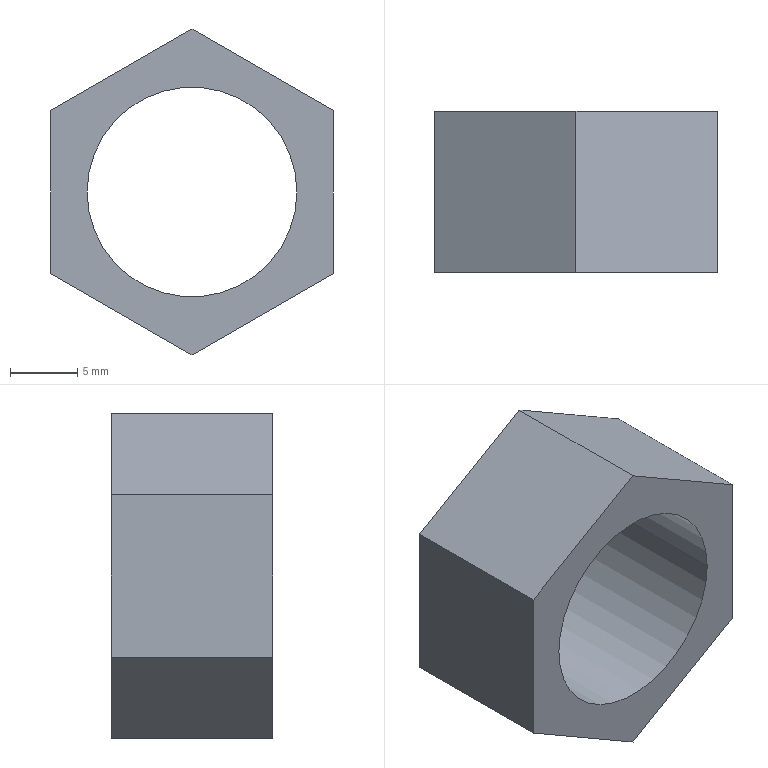Part | STEP file | Scale factor 1[13] | 1 solid | 10 faces | box 21 x 12 x 24.249 mm | volume 2289 mm3 | plane 8 | cylinder 2 | commonest cylinder face diameters 15.6 x2
STEP:
#1=CARTESIAN_POINT('',(-666.538,-401.273,3148.5));
#2=VERTEX_POINT('',#1);
#3=CARTESIAN_POINT('',(-650.938,-401.273,3148.5));
#4=VERTEX_POINT('',#3);
#5=CARTESIAN_POINT('',(-658.738,-401.273,3148.5));
#6=DIRECTION('',(0.,1.,0.));
#7=DIRECTION('',(1.,0.,0.000000001));
#8=AXIS2_PLACEMENT_3D('',#5,#6,#7);
#9=CIRCLE('',#8,7.8);
#10=EDGE_CURVE('',#2,#4,#9,.T.);
#11=ORIENTED_EDGE('',*,*,#10,.T.);
#12=CARTESIAN_POINT('',(-650.938,-413.273,3148.5));
#13=VERTEX_POINT('',#12);
#14=CARTESIAN_POINT('',(-650.938,-401.273,3148.5));
#15=DIRECTION('',(0.,1.,0.));
#16=VECTOR('',#15,1000.);
#17=LINE('',#14,#16);
#18=EDGE_CURVE('',#13,#4,#17,.T.);
#19=ORIENTED_EDGE('',*,*,#18,.F.);
#20=CARTESIAN_POINT('',(-666.538,-413.273,3148.5));
#21=VERTEX_POINT('',#20);
#22=CARTESIAN_POINT('',(-658.738,-413.273,3148.5));
#23=DIRECTION('',(0.,1.,0.));
#24=DIRECTION('',(1.,0.,0.000000001));
#25=AXIS2_PLACEMENT_3D('',#22,#23,#24);
#26=CIRCLE('',#25,7.8);
#27=EDGE_CURVE('',#21,#13,#26,.T.);
#28=ORIENTED_EDGE('',*,*,#27,.F.);
#29=CARTESIAN_POINT('',(-666.538,-401.273,3148.5));
#30=DIRECTION('',(0.,1.,0.));
#31=VECTOR('',#30,1000.);
#32=LINE('',#29,#31);
#33=EDGE_CURVE('',#21,#2,#32,.T.);
#34=ORIENTED_EDGE('',*,*,#33,.T.);
#35=EDGE_LOOP('',(#11,#19,#28,#34));
#36=FACE_OUTER_BOUND('',#35,.T.);
#37=CARTESIAN_POINT('',(-658.738,-401.273,3148.5));
#38=DIRECTION('',(0.,-1.,0.));
#39=DIRECTION('',(1.,0.,0.000000001));
#40=AXIS2_PLACEMENT_3D('',#37,#38,#39);
#41=CYLINDRICAL_SURFACE('',#40,7.8);
#42=ADVANCED_FACE('',(#36),#41,.F.);
#43=CARTESIAN_POINT('',(-648.238,-401.273,3142.438));
#44=VERTEX_POINT('',#43);
#45=CARTESIAN_POINT('',(-658.738,-401.273,3136.376));
#46=VERTEX_POINT('',#45);
#47=CARTESIAN_POINT('',(-648.238,-401.273,3142.438));
#48=DIRECTION('',(-0.866,0.,-0.5));
#49=VECTOR('',#48,1000.);
#50=LINE('',#47,#49);
#51=EDGE_CURVE('',#44,#46,#50,.T.);
#52=ORIENTED_EDGE('',*,*,#51,.T.);
#53=CARTESIAN_POINT('',(-669.238,-401.273,3142.438));
#54=VERTEX_POINT('',#53);
#55=CARTESIAN_POINT('',(-658.738,-401.273,3136.376));
#56=DIRECTION('',(-0.866,0.,0.5));
#57=VECTOR('',#56,1000.);
#58=LINE('',#55,#57);
#59=EDGE_CURVE('',#46,#54,#58,.T.);
#60=ORIENTED_EDGE('',*,*,#59,.T.);
#61=CARTESIAN_POINT('',(-669.238,-401.273,3154.562));
#62=VERTEX_POINT('',#61);
#63=CARTESIAN_POINT('',(-669.238,-401.273,3142.438));
#64=DIRECTION('',(-0.000000001,0.,1.));
#65=VECTOR('',#64,1000.);
#66=LINE('',#63,#65);
#67=EDGE_CURVE('',#54,#62,#66,.T.);
#68=ORIENTED_EDGE('',*,*,#67,.T.);
#69=CARTESIAN_POINT('',(-658.738,-401.273,3160.624));
#70=VERTEX_POINT('',#69);
#71=CARTESIAN_POINT('',(-669.238,-401.273,3154.562));
#72=DIRECTION('',(0.866,0.,0.5));
#73=VECTOR('',#72,1000.);
#74=LINE('',#71,#73);
#75=EDGE_CURVE('',#62,#70,#74,.T.);
#76=ORIENTED_EDGE('',*,*,#75,.T.);
#77=CARTESIAN_POINT('',(-648.238,-401.273,3154.562));
#78=VERTEX_POINT('',#77);
#79=CARTESIAN_POINT('',(-658.738,-401.273,3160.624));
#80=DIRECTION('',(0.866,0.,-0.5));
#81=VECTOR('',#80,1000.);
#82=LINE('',#79,#81);
#83=EDGE_CURVE('',#70,#78,#82,.T.);
#84=ORIENTED_EDGE('',*,*,#83,.T.);
#85=CARTESIAN_POINT('',(-648.238,-401.273,3154.562));
#86=DIRECTION('',(0.000000001,0.,-1.));
#87=VECTOR('',#86,1000.);
#88=LINE('',#85,#87);
#89=EDGE_CURVE('',#78,#44,#88,.T.);
#90=ORIENTED_EDGE('',*,*,#89,.T.);
#91=EDGE_LOOP('',(#52,#60,#68,#76,#84,#90));
#92=FACE_OUTER_BOUND('',#91,.T.);
#93=ORIENTED_EDGE('',*,*,#10,.F.);
#94=CARTESIAN_POINT('',(-658.738,-401.273,3148.5));
#95=DIRECTION('',(0.,1.,0.));
#96=DIRECTION('',(1.,0.,0.000000001));
#97=AXIS2_PLACEMENT_3D('',#94,#95,#96);
#98=CIRCLE('',#97,7.8);
#99=EDGE_CURVE('',#4,#2,#98,.T.);
#100=ORIENTED_EDGE('',*,*,#99,.F.);
#101=EDGE_LOOP('',(#93,#100));
#102=FACE_BOUND('',#101,.T.);
#103=CARTESIAN_POINT('',(-658.738,-401.273,3148.5));
#104=DIRECTION('',(0.,1.,0.));
#105=DIRECTION('',(-1.,0.,-0.000000001));
#106=AXIS2_PLACEMENT_3D('',#103,#104,#105);
#107=PLANE('',#106);
#108=ADVANCED_FACE('',(#92,#102),#107,.T.);
#109=CARTESIAN_POINT('',(-648.238,-413.273,3142.438));
#110=VERTEX_POINT('',#109);
#111=CARTESIAN_POINT('',(-658.738,-413.273,3136.376));
#112=VERTEX_POINT('',#111);
#113=CARTESIAN_POINT('',(-648.238,-413.273,3142.438));
#114=DIRECTION('',(-0.866,0.,-0.5));
#115=VECTOR('',#114,1000.);
#116=LINE('',#113,#115);
#117=EDGE_CURVE('',#110,#112,#116,.T.);
#118=ORIENTED_EDGE('',*,*,#117,.F.);
#119=CARTESIAN_POINT('',(-648.238,-413.273,3154.562));
#120=VERTEX_POINT('',#119);
#121=CARTESIAN_POINT('',(-648.238,-413.273,3154.562));
#122=DIRECTION('',(0.000000001,0.,-1.));
#123=VECTOR('',#122,1000.);
#124=LINE('',#121,#123);
#125=EDGE_CURVE('',#120,#110,#124,.T.);
#126=ORIENTED_EDGE('',*,*,#125,.F.);
#127=CARTESIAN_POINT('',(-658.738,-413.273,3160.624));
#128=VERTEX_POINT('',#127);
#129=CARTESIAN_POINT('',(-658.738,-413.273,3160.624));
#130=DIRECTION('',(0.866,0.,-0.5));
#131=VECTOR('',#130,1000.);
#132=LINE('',#129,#131);
#133=EDGE_CURVE('',#128,#120,#132,.T.);
#134=ORIENTED_EDGE('',*,*,#133,.F.);
#135=CARTESIAN_POINT('',(-669.238,-413.273,3154.562));
#136=VERTEX_POINT('',#135);
#137=CARTESIAN_POINT('',(-669.238,-413.273,3154.562));
#138=DIRECTION('',(0.866,0.,0.5));
#139=VECTOR('',#138,1000.);
#140=LINE('',#137,#139);
#141=EDGE_CURVE('',#136,#128,#140,.T.);
#142=ORIENTED_EDGE('',*,*,#141,.F.);
#143=CARTESIAN_POINT('',(-669.238,-413.273,3142.438));
#144=VERTEX_POINT('',#143);
#145=CARTESIAN_POINT('',(-669.238,-413.273,3142.438));
#146=DIRECTION('',(-0.000000001,0.,1.));
#147=VECTOR('',#146,1000.);
#148=LINE('',#145,#147);
#149=EDGE_CURVE('',#144,#136,#148,.T.);
#150=ORIENTED_EDGE('',*,*,#149,.F.);
#151=CARTESIAN_POINT('',(-658.738,-413.273,3136.376));
#152=DIRECTION('',(-0.866,0.,0.5));
#153=VECTOR('',#152,1000.);
#154=LINE('',#151,#153);
#155=EDGE_CURVE('',#112,#144,#154,.T.);
#156=ORIENTED_EDGE('',*,*,#155,.F.);
#157=EDGE_LOOP('',(#118,#126,#134,#142,#150,#156));
#158=FACE_OUTER_BOUND('',#157,.T.);
#159=ORIENTED_EDGE('',*,*,#27,.T.);
#160=CARTESIAN_POINT('',(-658.738,-413.273,3148.5));
#161=DIRECTION('',(0.,1.,0.));
#162=DIRECTION('',(1.,0.,0.000000001));
#163=AXIS2_PLACEMENT_3D('',#160,#161,#162);
#164=CIRCLE('',#163,7.8);
#165=EDGE_CURVE('',#13,#21,#164,.T.);
#166=ORIENTED_EDGE('',*,*,#165,.T.);
#167=EDGE_LOOP('',(#159,#166));
#168=FACE_BOUND('',#167,.T.);
#169=CARTESIAN_POINT('',(-658.738,-413.273,3148.5));
#170=DIRECTION('',(0.,1.,0.));
#171=DIRECTION('',(-1.,0.,-0.000000001));
#172=AXIS2_PLACEMENT_3D('',#169,#170,#171);
#173=PLANE('',#172);
#174=ADVANCED_FACE('',(#158,#168),#173,.F.);
#175=ORIENTED_EDGE('',*,*,#117,.T.);
#176=CARTESIAN_POINT('',(-658.738,-401.273,3136.376));
#177=DIRECTION('',(0.,-1.,0.));
#178=VECTOR('',#177,1000.);
#179=LINE('',#176,#178);
#180=EDGE_CURVE('',#46,#112,#179,.T.);
#181=ORIENTED_EDGE('',*,*,#180,.F.);
#182=ORIENTED_EDGE('',*,*,#51,.F.);
#183=CARTESIAN_POINT('',(-648.238,-401.273,3142.438));
#184=DIRECTION('',(0.,-1.,0.));
#185=VECTOR('',#184,1000.);
#186=LINE('',#183,#185);
#187=EDGE_CURVE('',#44,#110,#186,.T.);
#188=ORIENTED_EDGE('',*,*,#187,.T.);
#189=EDGE_LOOP('',(#175,#181,#182,#188));
#190=FACE_OUTER_BOUND('',#189,.T.);
#191=CARTESIAN_POINT('',(-648.238,-401.273,3142.438));
#192=DIRECTION('',(-0.5,0.,0.866));
#193=DIRECTION('',(-0.866,0.,-0.5));
#194=AXIS2_PLACEMENT_3D('',#191,#192,#193);
#195=PLANE('',#194);
#196=ADVANCED_FACE('',(#190),#195,.F.);
#197=ORIENTED_EDGE('',*,*,#155,.T.);
#198=CARTESIAN_POINT('',(-669.238,-401.273,3142.438));
#199=DIRECTION('',(0.,-1.,0.));
#200=VECTOR('',#199,1000.);
#201=LINE('',#198,#200);
#202=EDGE_CURVE('',#54,#144,#201,.T.);
#203=ORIENTED_EDGE('',*,*,#202,.F.);
#204=ORIENTED_EDGE('',*,*,#59,.F.);
#205=ORIENTED_EDGE('',*,*,#180,.T.);
#206=EDGE_LOOP('',(#197,#203,#204,#205));
#207=FACE_OUTER_BOUND('',#206,.T.);
#208=CARTESIAN_POINT('',(-658.738,-401.273,3136.376));
#209=DIRECTION('',(0.5,0.,0.866));
#210=DIRECTION('',(-0.866,0.,0.5));
#211=AXIS2_PLACEMENT_3D('',#208,#209,#210);
#212=PLANE('',#211);
#213=ADVANCED_FACE('',(#207),#212,.F.);
#214=ORIENTED_EDGE('',*,*,#149,.T.);
#215=CARTESIAN_POINT('',(-669.238,-401.273,3154.562));
#216=DIRECTION('',(0.,-1.,0.));
#217=VECTOR('',#216,1000.);
#218=LINE('',#215,#217);
#219=EDGE_CURVE('',#62,#136,#218,.T.);
#220=ORIENTED_EDGE('',*,*,#219,.F.);
#221=ORIENTED_EDGE('',*,*,#67,.F.);
#222=ORIENTED_EDGE('',*,*,#202,.T.);
#223=EDGE_LOOP('',(#214,#220,#221,#222));
#224=FACE_OUTER_BOUND('',#223,.T.);
#225=CARTESIAN_POINT('',(-669.238,-401.273,3142.438));
#226=DIRECTION('',(1.,0.,0.000000001));
#227=DIRECTION('',(-0.000000001,0.,1.));
#228=AXIS2_PLACEMENT_3D('',#225,#226,#227);
#229=PLANE('',#228);
#230=ADVANCED_FACE('',(#224),#229,.F.);
#231=ORIENTED_EDGE('',*,*,#141,.T.);
#232=CARTESIAN_POINT('',(-658.738,-401.273,3160.624));
#233=DIRECTION('',(0.,-1.,0.));
#234=VECTOR('',#233,1000.);
#235=LINE('',#232,#234);
#236=EDGE_CURVE('',#70,#128,#235,.T.);
#237=ORIENTED_EDGE('',*,*,#236,.F.);
#238=ORIENTED_EDGE('',*,*,#75,.F.);
#239=ORIENTED_EDGE('',*,*,#219,.T.);
#240=EDGE_LOOP('',(#231,#237,#238,#239));
#241=FACE_OUTER_BOUND('',#240,.T.);
#242=CARTESIAN_POINT('',(-669.238,-401.273,3154.562));
#243=DIRECTION('',(0.5,0.,-0.866));
#244=DIRECTION('',(0.866,0.,0.5));
#245=AXIS2_PLACEMENT_3D('',#242,#243,#244);
#246=PLANE('',#245);
#247=ADVANCED_FACE('',(#241),#246,.F.);
#248=ORIENTED_EDGE('',*,*,#133,.T.);
#249=CARTESIAN_POINT('',(-648.238,-401.273,3154.562));
#250=DIRECTION('',(0.,-1.,0.));
#251=VECTOR('',#250,1000.);
#252=LINE('',#249,#251);
#253=EDGE_CURVE('',#78,#120,#252,.T.);
#254=ORIENTED_EDGE('',*,*,#253,.F.);
#255=ORIENTED_EDGE('',*,*,#83,.F.);
#256=ORIENTED_EDGE('',*,*,#236,.T.);
#257=EDGE_LOOP('',(#248,#254,#255,#256));
#258=FACE_OUTER_BOUND('',#257,.T.);
#259=CARTESIAN_POINT('',(-658.738,-401.273,3160.624));
#260=DIRECTION('',(-0.5,0.,-0.866));
#261=DIRECTION('',(0.866,0.,-0.5));
#262=AXIS2_PLACEMENT_3D('',#259,#260,#261);
#263=PLANE('',#262);
#264=ADVANCED_FACE('',(#258),#263,.F.);
#265=ORIENTED_EDGE('',*,*,#125,.T.);
#266=ORIENTED_EDGE('',*,*,#187,.F.);
#267=ORIENTED_EDGE('',*,*,#89,.F.);
#268=ORIENTED_EDGE('',*,*,#253,.T.);
#269=EDGE_LOOP('',(#265,#266,#267,#268));
#270=FACE_OUTER_BOUND('',#269,.T.);
#271=CARTESIAN_POINT('',(-648.238,-401.273,3154.562));
#272=DIRECTION('',(-1.,0.,-0.000000001));
#273=DIRECTION('',(0.000000001,0.,-1.));
#274=AXIS2_PLACEMENT_3D('',#271,#272,#273);
#275=PLANE('',#274);
#276=ADVANCED_FACE('',(#270),#275,.F.);
#277=ORIENTED_EDGE('',*,*,#18,.T.);
#278=ORIENTED_EDGE('',*,*,#99,.T.);
#279=ORIENTED_EDGE('',*,*,#33,.F.);
#280=ORIENTED_EDGE('',*,*,#165,.F.);
#281=EDGE_LOOP('',(#277,#278,#279,#280));
#282=FACE_OUTER_BOUND('',#281,.T.);
#283=CARTESIAN_POINT('',(-658.738,-401.273,3148.5));
#284=DIRECTION('',(0.,-1.,0.));
#285=DIRECTION('',(1.,0.,0.000000001));
#286=AXIS2_PLACEMENT_3D('',#283,#284,#285);
#287=CYLINDRICAL_SURFACE('',#286,7.8);
#288=ADVANCED_FACE('',(#282),#287,.F.);
#289=CLOSED_SHELL('',(#42,#108,#174,#196,#213,#230,#247,#264,#276,#288));
#290=MANIFOLD_SOLID_BREP('',#289);
#291=CARTESIAN_POINT('',(0.,0.,0.));
#292=DIRECTION('',(0.,0.,1.));
#293=DIRECTION('',(1.,0.,0.));
#294=AXIS2_PLACEMENT_3D('',#291,#292,#293);
#295=(LENGTH_UNIT()NAMED_UNIT(*)SI_UNIT(.MILLI.,.METRE.));
#296=UNCERTAINTY_MEASURE_WITH_UNIT(LENGTH_MEASURE(0.00001),#295,'','');
#297=(NAMED_UNIT(*)PLANE_ANGLE_UNIT()SI_UNIT($,.RADIAN.));
#298=(NAMED_UNIT(*)SI_UNIT($,.STERADIAN.)SOLID_ANGLE_UNIT());
#299=(GEOMETRIC_REPRESENTATION_CONTEXT(3)GLOBAL_UNCERTAINTY_ASSIGNED_CONTEXT((#296))GLOBAL_UNIT_ASSIGNED_CONTEXT((#295,#297,#298))REPRESENTATION_CONTEXT('',''));
#300=ADVANCED_BREP_SHAPE_REPRESENTATION('',(#290,#294),#299);